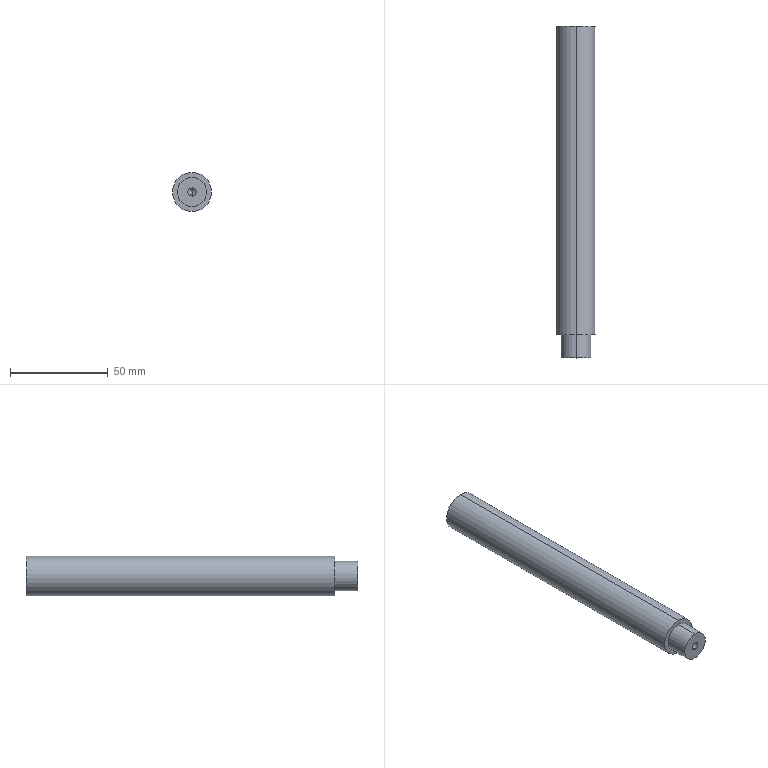Part | STEP file | 1 solid | 11 faces | box 20 x 170 x 20 mm | volume 51580 mm3 | cylinder 6 | plane 3 | cone 2 | commonest cylinder face diameters 4.2 x2 15 x2 20 x2
STEP:
#1=CARTESIAN_POINT('',(0.,0.,0.));
#2=DIRECTION('',(0.,0.,1.));
#3=DIRECTION('',(1.,0.,0.));
#4=AXIS2_PLACEMENT_3D('',#1,#2,#3);
#5=CARTESIAN_POINT('',(0.,12.4,-2.1));
#6=VERTEX_POINT('',#5);
#7=CARTESIAN_POINT('',(0.,0.,-2.1));
#8=VERTEX_POINT('',#7);
#9=CARTESIAN_POINT('',(0.,0.,-2.1));
#10=DIRECTION('',(0.,-1.,0.));
#11=VECTOR('',#10,1.);
#12=LINE('',#9,#11);
#13=CARTESIAN_POINT('',(0.,0.,0.));
#14=DIRECTION('',(0.,-1.,0.));
#15=DIRECTION('',(0.,0.,-1.));
#16=AXIS2_PLACEMENT_3D('',#13,#14,#15);
#17=CYLINDRICAL_SURFACE('',#16,2.1);
#18=CARTESIAN_POINT('',(6.283,0.));
#19=DIRECTION('',(0.,1.));
#20=VECTOR('',#19,1.);
#21=LINE('',#18,#20);
#22=(GEOMETRIC_REPRESENTATION_CONTEXT(2)PARAMETRIC_REPRESENTATION_CONTEXT()REPRESENTATION_CONTEXT('',''));
#23=DEFINITIONAL_REPRESENTATION('',(#21),#22);
#24=PCURVE('',#17,#23);
#25=CARTESIAN_POINT('',(0.,0.,0.));
#26=DIRECTION('',(0.,-1.,0.));
#27=DIRECTION('',(0.,0.,-1.));
#28=AXIS2_PLACEMENT_3D('',#25,#26,#27);
#29=CYLINDRICAL_SURFACE('',#28,2.1);
#30=CARTESIAN_POINT('',(0.,0.));
#31=DIRECTION('',(0.,1.));
#32=VECTOR('',#31,1.);
#33=LINE('',#30,#32);
#34=(GEOMETRIC_REPRESENTATION_CONTEXT(2)PARAMETRIC_REPRESENTATION_CONTEXT()REPRESENTATION_CONTEXT('',''));
#35=DEFINITIONAL_REPRESENTATION('',(#33),#34);
#36=PCURVE('',#29,#35);
#37=SURFACE_CURVE('',#12,(#24,#36),.PCURVE_S1.);
#38=EDGE_CURVE('',#6,#8,#37,.T.);
#39=ORIENTED_EDGE('',*,*,#38,.T.);
#40=CARTESIAN_POINT('',(0.,0.,2.1));
#41=VERTEX_POINT('',#40);
#42=CARTESIAN_POINT('',(0.,0.,0.));
#43=DIRECTION('',(0.,-1.,0.));
#44=DIRECTION('',(0.,0.,-1.));
#45=AXIS2_PLACEMENT_3D('',#42,#43,#44);
#46=CIRCLE('',#45,2.1);
#47=CARTESIAN_POINT('',(0.,0.));
#48=DIRECTION('',(1.,0.));
#49=VECTOR('',#48,1.);
#50=LINE('',#47,#49);
#51=(GEOMETRIC_REPRESENTATION_CONTEXT(2)PARAMETRIC_REPRESENTATION_CONTEXT()REPRESENTATION_CONTEXT('',''));
#52=DEFINITIONAL_REPRESENTATION('',(#50),#51);
#53=PCURVE('',#17,#52);
#54=CARTESIAN_POINT('',(0.,0.,0.));
#55=DIRECTION('',(0.,-1.,0.));
#56=DIRECTION('',(0.,0.,-1.));
#57=AXIS2_PLACEMENT_3D('',#54,#55,#56);
#58=PLANE('',#57);
#59=CARTESIAN_POINT('',(0.,0.));
#60=DIRECTION('',(1.,0.));
#61=AXIS2_PLACEMENT_2D('',#59,#60);
#62=CIRCLE('',#61,2.1);
#63=(GEOMETRIC_REPRESENTATION_CONTEXT(2)PARAMETRIC_REPRESENTATION_CONTEXT()REPRESENTATION_CONTEXT('',''));
#64=DEFINITIONAL_REPRESENTATION('',(#62),#63);
#65=PCURVE('',#58,#64);
#66=SURFACE_CURVE('',#46,(#53,#65),.PCURVE_S1.);
#67=EDGE_CURVE('',#41,#8,#66,.T.);
#68=ORIENTED_EDGE('',*,*,#67,.F.);
#69=CARTESIAN_POINT('',(0.,12.4,2.1));
#70=VERTEX_POINT('',#69);
#71=CARTESIAN_POINT('',(0.,0.,2.1));
#72=DIRECTION('',(0.,-1.,0.));
#73=VECTOR('',#72,1.);
#74=LINE('',#71,#73);
#75=CARTESIAN_POINT('',(3.142,0.));
#76=DIRECTION('',(0.,1.));
#77=VECTOR('',#76,1.);
#78=LINE('',#75,#77);
#79=(GEOMETRIC_REPRESENTATION_CONTEXT(2)PARAMETRIC_REPRESENTATION_CONTEXT()REPRESENTATION_CONTEXT('',''));
#80=DEFINITIONAL_REPRESENTATION('',(#78),#79);
#81=PCURVE('',#17,#80);
#82=CARTESIAN_POINT('',(3.142,0.));
#83=DIRECTION('',(0.,1.));
#84=VECTOR('',#83,1.);
#85=LINE('',#82,#84);
#86=(GEOMETRIC_REPRESENTATION_CONTEXT(2)PARAMETRIC_REPRESENTATION_CONTEXT()REPRESENTATION_CONTEXT('',''));
#87=DEFINITIONAL_REPRESENTATION('',(#85),#86);
#88=PCURVE('',#29,#87);
#89=SURFACE_CURVE('',#74,(#81,#88),.PCURVE_S1.);
#90=EDGE_CURVE('',#70,#41,#89,.T.);
#91=ORIENTED_EDGE('',*,*,#90,.F.);
#92=CARTESIAN_POINT('',(0.,12.4,0.));
#93=DIRECTION('',(0.,-1.,0.));
#94=DIRECTION('',(0.,0.,-1.));
#95=AXIS2_PLACEMENT_3D('',#92,#93,#94);
#96=CIRCLE('',#95,2.1);
#97=CARTESIAN_POINT('',(0.,-12.4));
#98=DIRECTION('',(1.,0.));
#99=VECTOR('',#98,1.);
#100=LINE('',#97,#99);
#101=(GEOMETRIC_REPRESENTATION_CONTEXT(2)PARAMETRIC_REPRESENTATION_CONTEXT()REPRESENTATION_CONTEXT('',''));
#102=DEFINITIONAL_REPRESENTATION('',(#100),#101);
#103=PCURVE('',#17,#102);
#104=CARTESIAN_POINT('',(0.,12.4,0.));
#105=DIRECTION('',(0.,-1.,0.));
#106=DIRECTION('',(0.,0.,-1.));
#107=AXIS2_PLACEMENT_3D('',#104,#105,#106);
#108=CONICAL_SURFACE('',#107,2.1,1.03);
#109=CARTESIAN_POINT('',(0.,0.));
#110=DIRECTION('',(1.,0.));
#111=VECTOR('',#110,1.);
#112=LINE('',#109,#111);
#113=(GEOMETRIC_REPRESENTATION_CONTEXT(2)PARAMETRIC_REPRESENTATION_CONTEXT()REPRESENTATION_CONTEXT('',''));
#114=DEFINITIONAL_REPRESENTATION('',(#112),#113);
#115=PCURVE('',#108,#114);
#116=SURFACE_CURVE('',#96,(#103,#115),.PCURVE_S1.);
#117=EDGE_CURVE('',#70,#6,#116,.T.);
#118=ORIENTED_EDGE('',*,*,#117,.T.);
#119=EDGE_LOOP('',(#39,#68,#91,#118));
#120=FACE_BOUND('',#119,.F.);
#121=ADVANCED_FACE('',(#120),#17,.F.);
#122=ORIENTED_EDGE('',*,*,#117,.F.);
#123=CARTESIAN_POINT('',(0.,13.662,0.));
#124=VERTEX_POINT('',#123);
#125=CARTESIAN_POINT('',(0.,12.4,2.1));
#126=DIRECTION('',(0.,-0.515,0.8572));
#127=VECTOR('',#126,1.);
#128=LINE('',#125,#127);
#129=CARTESIAN_POINT('',(3.142,0.));
#130=DIRECTION('',(0.,1.));
#131=VECTOR('',#130,1.);
#132=LINE('',#129,#131);
#133=(GEOMETRIC_REPRESENTATION_CONTEXT(2)PARAMETRIC_REPRESENTATION_CONTEXT()REPRESENTATION_CONTEXT('',''));
#134=DEFINITIONAL_REPRESENTATION('',(#132),#133);
#135=PCURVE('',#108,#134);
#136=CARTESIAN_POINT('',(0.,12.4,0.));
#137=DIRECTION('',(0.,-1.,0.));
#138=DIRECTION('',(0.,0.,-1.));
#139=AXIS2_PLACEMENT_3D('',#136,#137,#138);
#140=CONICAL_SURFACE('',#139,2.1,1.03);
#141=CARTESIAN_POINT('',(3.142,0.));
#142=DIRECTION('',(0.,1.));
#143=VECTOR('',#142,1.);
#144=LINE('',#141,#143);
#145=(GEOMETRIC_REPRESENTATION_CONTEXT(2)PARAMETRIC_REPRESENTATION_CONTEXT()REPRESENTATION_CONTEXT('',''));
#146=DEFINITIONAL_REPRESENTATION('',(#144),#145);
#147=PCURVE('',#140,#146);
#148=SURFACE_CURVE('',#128,(#135,#147),.PCURVE_S1.);
#149=EDGE_CURVE('',#124,#70,#148,.T.);
#150=ORIENTED_EDGE('',*,*,#149,.F.);
#151=CARTESIAN_POINT('',(0.,12.4,-2.1));
#152=DIRECTION('',(0.,-0.515,-0.8572));
#153=VECTOR('',#152,1.);
#154=LINE('',#151,#153);
#155=CARTESIAN_POINT('',(6.283,0.));
#156=DIRECTION('',(0.,1.));
#157=VECTOR('',#156,1.);
#158=LINE('',#155,#157);
#159=(GEOMETRIC_REPRESENTATION_CONTEXT(2)PARAMETRIC_REPRESENTATION_CONTEXT()REPRESENTATION_CONTEXT('',''));
#160=DEFINITIONAL_REPRESENTATION('',(#158),#159);
#161=PCURVE('',#108,#160);
#162=CARTESIAN_POINT('',(0.,0.));
#163=DIRECTION('',(0.,1.));
#164=VECTOR('',#163,1.);
#165=LINE('',#162,#164);
#166=(GEOMETRIC_REPRESENTATION_CONTEXT(2)PARAMETRIC_REPRESENTATION_CONTEXT()REPRESENTATION_CONTEXT('',''));
#167=DEFINITIONAL_REPRESENTATION('',(#165),#166);
#168=PCURVE('',#140,#167);
#169=SURFACE_CURVE('',#154,(#161,#168),.PCURVE_S1.);
#170=EDGE_CURVE('',#124,#6,#169,.T.);
#171=ORIENTED_EDGE('',*,*,#170,.T.);
#172=EDGE_LOOP('',(#122,#150,#171));
#173=FACE_BOUND('',#172,.F.);
#174=ADVANCED_FACE('',(#173),#108,.F.);
#175=CARTESIAN_POINT('',(0.,170.,-10.));
#176=VERTEX_POINT('',#175);
#177=CARTESIAN_POINT('',(0.,170.,10.));
#178=VERTEX_POINT('',#177);
#179=CARTESIAN_POINT('',(0.,170.,0.));
#180=DIRECTION('',(0.,-1.,0.));
#181=DIRECTION('',(0.,0.,-1.));
#182=AXIS2_PLACEMENT_3D('',#179,#180,#181);
#183=CIRCLE('',#182,10.);
#184=CARTESIAN_POINT('',(0.,0.,0.));
#185=DIRECTION('',(0.,-1.,0.));
#186=DIRECTION('',(0.,0.,-1.));
#187=AXIS2_PLACEMENT_3D('',#184,#185,#186);
#188=CYLINDRICAL_SURFACE('',#187,10.);
#189=CARTESIAN_POINT('',(0.,-170.));
#190=DIRECTION('',(1.,0.));
#191=VECTOR('',#190,1.);
#192=LINE('',#189,#191);
#193=(GEOMETRIC_REPRESENTATION_CONTEXT(2)PARAMETRIC_REPRESENTATION_CONTEXT()REPRESENTATION_CONTEXT('',''));
#194=DEFINITIONAL_REPRESENTATION('',(#192),#193);
#195=PCURVE('',#188,#194);
#196=CARTESIAN_POINT('',(10.,170.,0.));
#197=DIRECTION('',(0.,1.,0.));
#198=DIRECTION('',(0.,0.,1.));
#199=AXIS2_PLACEMENT_3D('',#196,#197,#198);
#200=PLANE('',#199);
#201=CARTESIAN_POINT('',(-10.,-10.));
#202=CARTESIAN_POINT('',(-10.,7.321));
#203=CARTESIAN_POINT('',(5.,-1.34));
#204=CARTESIAN_POINT('',(20.,-10.));
#205=CARTESIAN_POINT('',(5.,-18.66));
#206=CARTESIAN_POINT('',(-10.,-27.321));
#207=CARTESIAN_POINT('',(-10.,-10.));
#208=(BOUNDED_CURVE()B_SPLINE_CURVE(2,(#201,#202,#203,#204,#205,#206,#207),.UNSPECIFIED.,.T.,.F.)B_SPLINE_CURVE_WITH_KNOTS((1,2,2,2,2,1),(-2.094,0.,2.094,4.189,6.283,8.378),.UNSPECIFIED.)CURVE()GEOMETRIC_REPRESENTATION_ITEM()RATIONAL_B_SPLINE_CURVE((1.,0.5,1.,0.5,1.,0.5,1.))REPRESENTATION_ITEM(''));
#209=(GEOMETRIC_REPRESENTATION_CONTEXT(2)PARAMETRIC_REPRESENTATION_CONTEXT()REPRESENTATION_CONTEXT('',''));
#210=DEFINITIONAL_REPRESENTATION('',(#208),#209);
#211=PCURVE('',#200,#210);
#212=SURFACE_CURVE('',#183,(#195,#211),.PCURVE_S1.);
#213=EDGE_CURVE('',#176,#178,#212,.T.);
#214=ORIENTED_EDGE('',*,*,#213,.T.);
#215=CARTESIAN_POINT('',(0.,12.,10.));
#216=VERTEX_POINT('',#215);
#217=CARTESIAN_POINT('',(0.,0.,10.));
#218=DIRECTION('',(0.,-1.,0.));
#219=VECTOR('',#218,1.);
#220=LINE('',#217,#219);
#221=CARTESIAN_POINT('',(3.142,0.));
#222=DIRECTION('',(0.,1.));
#223=VECTOR('',#222,1.);
#224=LINE('',#221,#223);
#225=(GEOMETRIC_REPRESENTATION_CONTEXT(2)PARAMETRIC_REPRESENTATION_CONTEXT()REPRESENTATION_CONTEXT('',''));
#226=DEFINITIONAL_REPRESENTATION('',(#224),#225);
#227=PCURVE('',#188,#226);
#228=CARTESIAN_POINT('',(0.,0.,0.));
#229=DIRECTION('',(0.,-1.,0.));
#230=DIRECTION('',(0.,0.,-1.));
#231=AXIS2_PLACEMENT_3D('',#228,#229,#230);
#232=CYLINDRICAL_SURFACE('',#231,10.);
#233=CARTESIAN_POINT('',(3.142,0.));
#234=DIRECTION('',(0.,1.));
#235=VECTOR('',#234,1.);
#236=LINE('',#233,#235);
#237=(GEOMETRIC_REPRESENTATION_CONTEXT(2)PARAMETRIC_REPRESENTATION_CONTEXT()REPRESENTATION_CONTEXT('',''));
#238=DEFINITIONAL_REPRESENTATION('',(#236),#237);
#239=PCURVE('',#232,#238);
#240=SURFACE_CURVE('',#220,(#227,#239),.PCURVE_S1.);
#241=EDGE_CURVE('',#178,#216,#240,.T.);
#242=ORIENTED_EDGE('',*,*,#241,.T.);
#243=CARTESIAN_POINT('',(0.,12.,-10.));
#244=VERTEX_POINT('',#243);
#245=CARTESIAN_POINT('',(0.,12.,0.));
#246=DIRECTION('',(0.,-1.,0.));
#247=DIRECTION('',(0.,0.,-1.));
#248=AXIS2_PLACEMENT_3D('',#245,#246,#247);
#249=CIRCLE('',#248,10.);
#250=CARTESIAN_POINT('',(0.,-12.));
#251=DIRECTION('',(1.,0.));
#252=VECTOR('',#251,1.);
#253=LINE('',#250,#252);
#254=(GEOMETRIC_REPRESENTATION_CONTEXT(2)PARAMETRIC_REPRESENTATION_CONTEXT()REPRESENTATION_CONTEXT('',''));
#255=DEFINITIONAL_REPRESENTATION('',(#253),#254);
#256=PCURVE('',#188,#255);
#257=CARTESIAN_POINT('',(7.5,12.,0.));
#258=DIRECTION('',(0.,-1.,0.));
#259=DIRECTION('',(0.,0.,-1.));
#260=AXIS2_PLACEMENT_3D('',#257,#258,#259);
#261=PLANE('',#260);
#262=CARTESIAN_POINT('',(0.,-7.5));
#263=DIRECTION('',(1.,0.));
#264=AXIS2_PLACEMENT_2D('',#262,#263);
#265=CIRCLE('',#264,10.);
#266=(GEOMETRIC_REPRESENTATION_CONTEXT(2)PARAMETRIC_REPRESENTATION_CONTEXT()REPRESENTATION_CONTEXT('',''));
#267=DEFINITIONAL_REPRESENTATION('',(#265),#266);
#268=PCURVE('',#261,#267);
#269=SURFACE_CURVE('',#249,(#256,#268),.PCURVE_S1.);
#270=EDGE_CURVE('',#244,#216,#269,.T.);
#271=ORIENTED_EDGE('',*,*,#270,.F.);
#272=CARTESIAN_POINT('',(0.,0.,-10.));
#273=DIRECTION('',(0.,-1.,0.));
#274=VECTOR('',#273,1.);
#275=LINE('',#272,#274);
#276=CARTESIAN_POINT('',(0.,0.));
#277=DIRECTION('',(0.,1.));
#278=VECTOR('',#277,1.);
#279=LINE('',#276,#278);
#280=(GEOMETRIC_REPRESENTATION_CONTEXT(2)PARAMETRIC_REPRESENTATION_CONTEXT()REPRESENTATION_CONTEXT('',''));
#281=DEFINITIONAL_REPRESENTATION('',(#279),#280);
#282=PCURVE('',#188,#281);
#283=CARTESIAN_POINT('',(6.283,0.));
#284=DIRECTION('',(0.,1.));
#285=VECTOR('',#284,1.);
#286=LINE('',#283,#285);
#287=(GEOMETRIC_REPRESENTATION_CONTEXT(2)PARAMETRIC_REPRESENTATION_CONTEXT()REPRESENTATION_CONTEXT('',''));
#288=DEFINITIONAL_REPRESENTATION('',(#286),#287);
#289=PCURVE('',#232,#288);
#290=SURFACE_CURVE('',#275,(#282,#289),.PCURVE_S1.);
#291=EDGE_CURVE('',#176,#244,#290,.T.);
#292=ORIENTED_EDGE('',*,*,#291,.F.);
#293=EDGE_LOOP('',(#214,#242,#271,#292));
#294=FACE_BOUND('',#293,.T.);
#295=ADVANCED_FACE('',(#294),#188,.T.);
#296=CARTESIAN_POINT('',(0.,12.,-7.5));
#297=VERTEX_POINT('',#296);
#298=CARTESIAN_POINT('',(0.,12.,7.5));
#299=VERTEX_POINT('',#298);
#300=CARTESIAN_POINT('',(0.,12.,0.));
#301=DIRECTION('',(0.,-1.,0.));
#302=DIRECTION('',(0.,0.,-1.));
#303=AXIS2_PLACEMENT_3D('',#300,#301,#302);
#304=CIRCLE('',#303,7.5);
#305=CARTESIAN_POINT('',(0.,0.,0.));
#306=DIRECTION('',(0.,-1.,0.));
#307=DIRECTION('',(0.,0.,-1.));
#308=AXIS2_PLACEMENT_3D('',#305,#306,#307);
#309=CYLINDRICAL_SURFACE('',#308,7.5);
#310=CARTESIAN_POINT('',(0.,-12.));
#311=DIRECTION('',(1.,0.));
#312=VECTOR('',#311,1.);
#313=LINE('',#310,#312);
#314=(GEOMETRIC_REPRESENTATION_CONTEXT(2)PARAMETRIC_REPRESENTATION_CONTEXT()REPRESENTATION_CONTEXT('',''));
#315=DEFINITIONAL_REPRESENTATION('',(#313),#314);
#316=PCURVE('',#309,#315);
#317=CARTESIAN_POINT('',(0.,-7.5));
#318=DIRECTION('',(1.,0.));
#319=AXIS2_PLACEMENT_2D('',#317,#318);
#320=CIRCLE('',#319,7.5);
#321=(GEOMETRIC_REPRESENTATION_CONTEXT(2)PARAMETRIC_REPRESENTATION_CONTEXT()REPRESENTATION_CONTEXT('',''));
#322=DEFINITIONAL_REPRESENTATION('',(#320),#321);
#323=PCURVE('',#261,#322);
#324=SURFACE_CURVE('',#304,(#316,#323),.PCURVE_S1.);
#325=EDGE_CURVE('',#297,#299,#324,.T.);
#326=ORIENTED_EDGE('',*,*,#325,.T.);
#327=CARTESIAN_POINT('',(0.,0.,7.5));
#328=VERTEX_POINT('',#327);
#329=CARTESIAN_POINT('',(0.,0.,7.5));
#330=DIRECTION('',(0.,-1.,0.));
#331=VECTOR('',#330,1.);
#332=LINE('',#329,#331);
#333=CARTESIAN_POINT('',(3.142,0.));
#334=DIRECTION('',(0.,1.));
#335=VECTOR('',#334,1.);
#336=LINE('',#333,#335);
#337=(GEOMETRIC_REPRESENTATION_CONTEXT(2)PARAMETRIC_REPRESENTATION_CONTEXT()REPRESENTATION_CONTEXT('',''));
#338=DEFINITIONAL_REPRESENTATION('',(#336),#337);
#339=PCURVE('',#309,#338);
#340=CARTESIAN_POINT('',(0.,0.,0.));
#341=DIRECTION('',(0.,-1.,0.));
#342=DIRECTION('',(0.,0.,-1.));
#343=AXIS2_PLACEMENT_3D('',#340,#341,#342);
#344=CYLINDRICAL_SURFACE('',#343,7.5);
#345=CARTESIAN_POINT('',(3.142,0.));
#346=DIRECTION('',(0.,1.));
#347=VECTOR('',#346,1.);
#348=LINE('',#345,#347);
#349=(GEOMETRIC_REPRESENTATION_CONTEXT(2)PARAMETRIC_REPRESENTATION_CONTEXT()REPRESENTATION_CONTEXT('',''));
#350=DEFINITIONAL_REPRESENTATION('',(#348),#349);
#351=PCURVE('',#344,#350);
#352=SURFACE_CURVE('',#332,(#339,#351),.PCURVE_S1.);
#353=EDGE_CURVE('',#299,#328,#352,.T.);
#354=ORIENTED_EDGE('',*,*,#353,.T.);
#355=CARTESIAN_POINT('',(0.,0.,-7.5));
#356=VERTEX_POINT('',#355);
#357=CARTESIAN_POINT('',(0.,0.,0.));
#358=DIRECTION('',(0.,-1.,0.));
#359=DIRECTION('',(0.,0.,-1.));
#360=AXIS2_PLACEMENT_3D('',#357,#358,#359);
#361=CIRCLE('',#360,7.5);
#362=CARTESIAN_POINT('',(0.,0.));
#363=DIRECTION('',(1.,0.));
#364=VECTOR('',#363,1.);
#365=LINE('',#362,#364);
#366=(GEOMETRIC_REPRESENTATION_CONTEXT(2)PARAMETRIC_REPRESENTATION_CONTEXT()REPRESENTATION_CONTEXT('',''));
#367=DEFINITIONAL_REPRESENTATION('',(#365),#366);
#368=PCURVE('',#309,#367);
#369=CARTESIAN_POINT('',(0.,0.));
#370=DIRECTION('',(1.,0.));
#371=AXIS2_PLACEMENT_2D('',#369,#370);
#372=CIRCLE('',#371,7.5);
#373=(GEOMETRIC_REPRESENTATION_CONTEXT(2)PARAMETRIC_REPRESENTATION_CONTEXT()REPRESENTATION_CONTEXT('',''));
#374=DEFINITIONAL_REPRESENTATION('',(#372),#373);
#375=PCURVE('',#58,#374);
#376=SURFACE_CURVE('',#361,(#368,#375),.PCURVE_S1.);
#377=EDGE_CURVE('',#356,#328,#376,.T.);
#378=ORIENTED_EDGE('',*,*,#377,.F.);
#379=CARTESIAN_POINT('',(0.,0.,-7.5));
#380=DIRECTION('',(0.,-1.,0.));
#381=VECTOR('',#380,1.);
#382=LINE('',#379,#381);
#383=CARTESIAN_POINT('',(0.,0.));
#384=DIRECTION('',(0.,1.));
#385=VECTOR('',#384,1.);
#386=LINE('',#383,#385);
#387=(GEOMETRIC_REPRESENTATION_CONTEXT(2)PARAMETRIC_REPRESENTATION_CONTEXT()REPRESENTATION_CONTEXT('',''));
#388=DEFINITIONAL_REPRESENTATION('',(#386),#387);
#389=PCURVE('',#309,#388);
#390=CARTESIAN_POINT('',(6.283,0.));
#391=DIRECTION('',(0.,1.));
#392=VECTOR('',#391,1.);
#393=LINE('',#390,#392);
#394=(GEOMETRIC_REPRESENTATION_CONTEXT(2)PARAMETRIC_REPRESENTATION_CONTEXT()REPRESENTATION_CONTEXT('',''));
#395=DEFINITIONAL_REPRESENTATION('',(#393),#394);
#396=PCURVE('',#344,#395);
#397=SURFACE_CURVE('',#382,(#389,#396),.PCURVE_S1.);
#398=EDGE_CURVE('',#297,#356,#397,.T.);
#399=ORIENTED_EDGE('',*,*,#398,.F.);
#400=EDGE_LOOP('',(#326,#354,#378,#399));
#401=FACE_BOUND('',#400,.T.);
#402=ADVANCED_FACE('',(#401),#309,.T.);
#403=CARTESIAN_POINT('',(0.,0.,0.));
#404=DIRECTION('',(0.,-1.,0.));
#405=DIRECTION('',(0.,0.,-1.));
#406=AXIS2_PLACEMENT_3D('',#403,#404,#405);
#407=CIRCLE('',#406,2.1);
#408=CARTESIAN_POINT('',(0.,0.));
#409=DIRECTION('',(1.,0.));
#410=AXIS2_PLACEMENT_2D('',#408,#409);
#411=CIRCLE('',#410,2.1);
#412=(GEOMETRIC_REPRESENTATION_CONTEXT(2)PARAMETRIC_REPRESENTATION_CONTEXT()REPRESENTATION_CONTEXT('',''));
#413=DEFINITIONAL_REPRESENTATION('',(#411),#412);
#414=PCURVE('',#58,#413);
#415=CARTESIAN_POINT('',(0.,0.));
#416=DIRECTION('',(1.,0.));
#417=VECTOR('',#416,1.);
#418=LINE('',#415,#417);
#419=(GEOMETRIC_REPRESENTATION_CONTEXT(2)PARAMETRIC_REPRESENTATION_CONTEXT()REPRESENTATION_CONTEXT('',''));
#420=DEFINITIONAL_REPRESENTATION('',(#418),#419);
#421=PCURVE('',#29,#420);
#422=SURFACE_CURVE('',#407,(#414,#421),.PCURVE_S1.);
#423=EDGE_CURVE('',#8,#41,#422,.T.);
#424=ORIENTED_EDGE('',*,*,#423,.F.);
#425=ORIENTED_EDGE('',*,*,#67,.F.);
#426=EDGE_LOOP('',(#424,#425));
#427=FACE_BOUND('',#426,.T.);
#428=ORIENTED_EDGE('',*,*,#377,.T.);
#429=CARTESIAN_POINT('',(0.,0.,0.));
#430=DIRECTION('',(0.,-1.,0.));
#431=DIRECTION('',(0.,0.,-1.));
#432=AXIS2_PLACEMENT_3D('',#429,#430,#431);
#433=CIRCLE('',#432,7.5);
#434=CARTESIAN_POINT('',(0.,0.));
#435=DIRECTION('',(1.,0.));
#436=AXIS2_PLACEMENT_2D('',#434,#435);
#437=CIRCLE('',#436,7.5);
#438=(GEOMETRIC_REPRESENTATION_CONTEXT(2)PARAMETRIC_REPRESENTATION_CONTEXT()REPRESENTATION_CONTEXT('',''));
#439=DEFINITIONAL_REPRESENTATION('',(#437),#438);
#440=PCURVE('',#58,#439);
#441=CARTESIAN_POINT('',(0.,0.));
#442=DIRECTION('',(1.,0.));
#443=VECTOR('',#442,1.);
#444=LINE('',#441,#443);
#445=(GEOMETRIC_REPRESENTATION_CONTEXT(2)PARAMETRIC_REPRESENTATION_CONTEXT()REPRESENTATION_CONTEXT('',''));
#446=DEFINITIONAL_REPRESENTATION('',(#444),#445);
#447=PCURVE('',#344,#446);
#448=SURFACE_CURVE('',#433,(#440,#447),.PCURVE_S1.);
#449=EDGE_CURVE('',#328,#356,#448,.T.);
#450=ORIENTED_EDGE('',*,*,#449,.T.);
#451=EDGE_LOOP('',(#428,#450));
#452=FACE_BOUND('',#451,.T.);
#453=ADVANCED_FACE('',(#427,#452),#58,.T.);
#454=ORIENTED_EDGE('',*,*,#353,.F.);
#455=CARTESIAN_POINT('',(0.,12.,0.));
#456=DIRECTION('',(0.,-1.,0.));
#457=DIRECTION('',(0.,0.,-1.));
#458=AXIS2_PLACEMENT_3D('',#455,#456,#457);
#459=CIRCLE('',#458,7.5);
#460=CARTESIAN_POINT('',(0.,-12.));
#461=DIRECTION('',(1.,0.));
#462=VECTOR('',#461,1.);
#463=LINE('',#460,#462);
#464=(GEOMETRIC_REPRESENTATION_CONTEXT(2)PARAMETRIC_REPRESENTATION_CONTEXT()REPRESENTATION_CONTEXT('',''));
#465=DEFINITIONAL_REPRESENTATION('',(#463),#464);
#466=PCURVE('',#344,#465);
#467=CARTESIAN_POINT('',(0.,-7.5));
#468=DIRECTION('',(1.,0.));
#469=AXIS2_PLACEMENT_2D('',#467,#468);
#470=CIRCLE('',#469,7.5);
#471=(GEOMETRIC_REPRESENTATION_CONTEXT(2)PARAMETRIC_REPRESENTATION_CONTEXT()REPRESENTATION_CONTEXT('',''));
#472=DEFINITIONAL_REPRESENTATION('',(#470),#471);
#473=PCURVE('',#261,#472);
#474=SURFACE_CURVE('',#459,(#466,#473),.PCURVE_S1.);
#475=EDGE_CURVE('',#299,#297,#474,.T.);
#476=ORIENTED_EDGE('',*,*,#475,.T.);
#477=ORIENTED_EDGE('',*,*,#398,.T.);
#478=ORIENTED_EDGE('',*,*,#449,.F.);
#479=EDGE_LOOP('',(#454,#476,#477,#478));
#480=FACE_BOUND('',#479,.T.);
#481=ADVANCED_FACE('',(#480),#344,.T.);
#482=ORIENTED_EDGE('',*,*,#270,.T.);
#483=CARTESIAN_POINT('',(0.,12.,0.));
#484=DIRECTION('',(0.,-1.,0.));
#485=DIRECTION('',(0.,0.,-1.));
#486=AXIS2_PLACEMENT_3D('',#483,#484,#485);
#487=CIRCLE('',#486,10.);
#488=CARTESIAN_POINT('',(0.,-7.5));
#489=DIRECTION('',(1.,0.));
#490=AXIS2_PLACEMENT_2D('',#488,#489);
#491=CIRCLE('',#490,10.);
#492=(GEOMETRIC_REPRESENTATION_CONTEXT(2)PARAMETRIC_REPRESENTATION_CONTEXT()REPRESENTATION_CONTEXT('',''));
#493=DEFINITIONAL_REPRESENTATION('',(#491),#492);
#494=PCURVE('',#261,#493);
#495=CARTESIAN_POINT('',(0.,-12.));
#496=DIRECTION('',(1.,0.));
#497=VECTOR('',#496,1.);
#498=LINE('',#495,#497);
#499=(GEOMETRIC_REPRESENTATION_CONTEXT(2)PARAMETRIC_REPRESENTATION_CONTEXT()REPRESENTATION_CONTEXT('',''));
#500=DEFINITIONAL_REPRESENTATION('',(#498),#499);
#501=PCURVE('',#232,#500);
#502=SURFACE_CURVE('',#487,(#494,#501),.PCURVE_S1.);
#503=EDGE_CURVE('',#216,#244,#502,.T.);
#504=ORIENTED_EDGE('',*,*,#503,.T.);
#505=EDGE_LOOP('',(#482,#504));
#506=FACE_BOUND('',#505,.T.);
#507=ORIENTED_EDGE('',*,*,#325,.F.);
#508=ORIENTED_EDGE('',*,*,#475,.F.);
#509=EDGE_LOOP('',(#507,#508));
#510=FACE_BOUND('',#509,.T.);
#511=ADVANCED_FACE('',(#506,#510),#261,.T.);
#512=ORIENTED_EDGE('',*,*,#241,.F.);
#513=CARTESIAN_POINT('',(0.,170.,0.));
#514=DIRECTION('',(0.,-1.,0.));
#515=DIRECTION('',(0.,0.,-1.));
#516=AXIS2_PLACEMENT_3D('',#513,#514,#515);
#517=CIRCLE('',#516,10.);
#518=CARTESIAN_POINT('',(0.,-170.));
#519=DIRECTION('',(1.,0.));
#520=VECTOR('',#519,1.);
#521=LINE('',#518,#520);
#522=(GEOMETRIC_REPRESENTATION_CONTEXT(2)PARAMETRIC_REPRESENTATION_CONTEXT()REPRESENTATION_CONTEXT('',''));
#523=DEFINITIONAL_REPRESENTATION('',(#521),#522);
#524=PCURVE('',#232,#523);
#525=CARTESIAN_POINT('',(-10.,-10.));
#526=CARTESIAN_POINT('',(-10.,7.321));
#527=CARTESIAN_POINT('',(5.,-1.34));
#528=CARTESIAN_POINT('',(20.,-10.));
#529=CARTESIAN_POINT('',(5.,-18.66));
#530=CARTESIAN_POINT('',(-10.,-27.321));
#531=CARTESIAN_POINT('',(-10.,-10.));
#532=(BOUNDED_CURVE()B_SPLINE_CURVE(2,(#525,#526,#527,#528,#529,#530,#531),.UNSPECIFIED.,.T.,.F.)B_SPLINE_CURVE_WITH_KNOTS((1,2,2,2,2,1),(-2.094,0.,2.094,4.189,6.283,8.378),.UNSPECIFIED.)CURVE()GEOMETRIC_REPRESENTATION_ITEM()RATIONAL_B_SPLINE_CURVE((1.,0.5,1.,0.5,1.,0.5,1.))REPRESENTATION_ITEM(''));
#533=(GEOMETRIC_REPRESENTATION_CONTEXT(2)PARAMETRIC_REPRESENTATION_CONTEXT()REPRESENTATION_CONTEXT('',''));
#534=DEFINITIONAL_REPRESENTATION('',(#532),#533);
#535=PCURVE('',#200,#534);
#536=SURFACE_CURVE('',#517,(#524,#535),.PCURVE_S1.);
#537=EDGE_CURVE('',#178,#176,#536,.T.);
#538=ORIENTED_EDGE('',*,*,#537,.T.);
#539=ORIENTED_EDGE('',*,*,#291,.T.);
#540=ORIENTED_EDGE('',*,*,#503,.F.);
#541=EDGE_LOOP('',(#512,#538,#539,#540));
#542=FACE_BOUND('',#541,.T.);
#543=ADVANCED_FACE('',(#542),#232,.T.);
#544=ORIENTED_EDGE('',*,*,#213,.F.);
#545=ORIENTED_EDGE('',*,*,#537,.F.);
#546=EDGE_LOOP('',(#544,#545));
#547=FACE_BOUND('',#546,.T.);
#548=ADVANCED_FACE('',(#547),#200,.T.);
#549=CARTESIAN_POINT('',(0.,12.4,0.));
#550=DIRECTION('',(0.,-1.,0.));
#551=DIRECTION('',(0.,0.,-1.));
#552=AXIS2_PLACEMENT_3D('',#549,#550,#551);
#553=CIRCLE('',#552,2.1);
#554=CARTESIAN_POINT('',(0.,0.));
#555=DIRECTION('',(1.,0.));
#556=VECTOR('',#555,1.);
#557=LINE('',#554,#556);
#558=(GEOMETRIC_REPRESENTATION_CONTEXT(2)PARAMETRIC_REPRESENTATION_CONTEXT()REPRESENTATION_CONTEXT('',''));
#559=DEFINITIONAL_REPRESENTATION('',(#557),#558);
#560=PCURVE('',#140,#559);
#561=CARTESIAN_POINT('',(0.,-12.4));
#562=DIRECTION('',(1.,0.));
#563=VECTOR('',#562,1.);
#564=LINE('',#561,#563);
#565=(GEOMETRIC_REPRESENTATION_CONTEXT(2)PARAMETRIC_REPRESENTATION_CONTEXT()REPRESENTATION_CONTEXT('',''));
#566=DEFINITIONAL_REPRESENTATION('',(#564),#565);
#567=PCURVE('',#29,#566);
#568=SURFACE_CURVE('',#553,(#560,#567),.PCURVE_S1.);
#569=EDGE_CURVE('',#6,#70,#568,.T.);
#570=ORIENTED_EDGE('',*,*,#569,.F.);
#571=ORIENTED_EDGE('',*,*,#170,.F.);
#572=ORIENTED_EDGE('',*,*,#149,.T.);
#573=EDGE_LOOP('',(#570,#571,#572));
#574=FACE_BOUND('',#573,.F.);
#575=ADVANCED_FACE('',(#574),#140,.F.);
#576=ORIENTED_EDGE('',*,*,#423,.F.);
#577=ORIENTED_EDGE('',*,*,#38,.F.);
#578=ORIENTED_EDGE('',*,*,#569,.T.);
#579=ORIENTED_EDGE('',*,*,#90,.T.);
#580=EDGE_LOOP('',(#576,#577,#578,#579));
#581=FACE_BOUND('',#580,.F.);
#582=ADVANCED_FACE('',(#581),#29,.F.);
#583=CLOSED_SHELL('',(#121,#174,#295,#402,#453,#481,#511,#543,#548,#575,#582));
#584=MANIFOLD_SOLID_BREP('',#583);
#585=(LENGTH_UNIT()NAMED_UNIT(*)SI_UNIT(.MILLI.,.METRE.));
#586=UNCERTAINTY_MEASURE_WITH_UNIT(LENGTH_MEASURE(0.0000001),#585,'','');
#587=(NAMED_UNIT(*)PLANE_ANGLE_UNIT()SI_UNIT($,.RADIAN.));
#588=(NAMED_UNIT(*)SI_UNIT($,.STERADIAN.)SOLID_ANGLE_UNIT());
#589=(GEOMETRIC_REPRESENTATION_CONTEXT(3)GLOBAL_UNCERTAINTY_ASSIGNED_CONTEXT((#586))GLOBAL_UNIT_ASSIGNED_CONTEXT((#585,#587,#588))REPRESENTATION_CONTEXT('',''));
#590=ADVANCED_BREP_SHAPE_REPRESENTATION('',(#4,#584),#589);